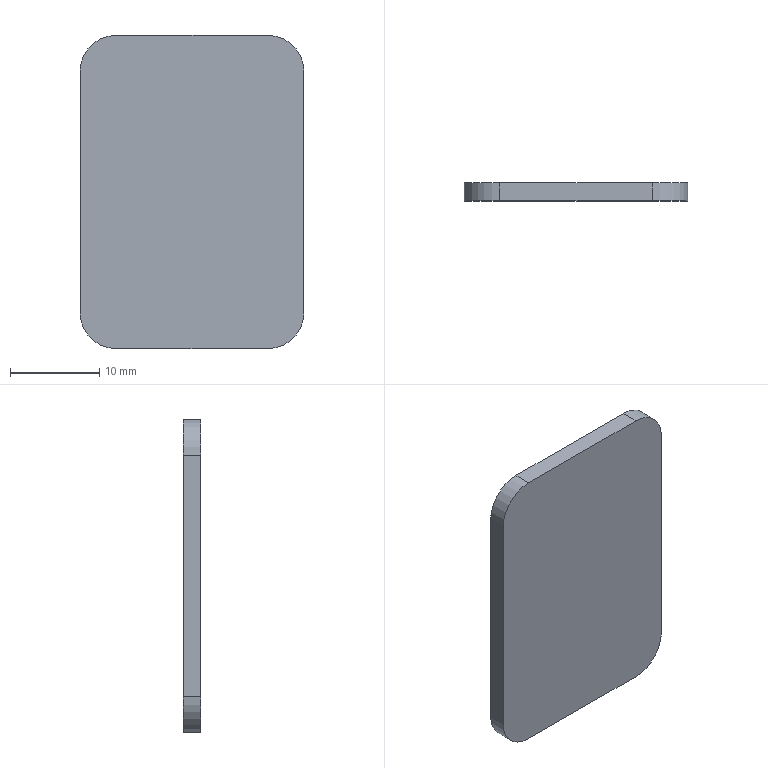Part | SolidWorks | features Extrusion 1 | 1 solid | 10 faces | box 25 x 2 x 35 mm | volume 1723 mm3 | plane 6 | cylinder 4 | commonest cylinder face diameters 8 x4
STEP:
#1=CARTESIAN_POINT('',(12.5,0.,-13.5));
#2=VERTEX_POINT('',#1);
#3=CARTESIAN_POINT('',(8.5,0.,-17.5));
#4=VERTEX_POINT('',#3);
#5=CARTESIAN_POINT('',(8.5,0.,-13.5));
#6=DIRECTION('',(0.,1.,0.));
#7=DIRECTION('',(0.,0.,1.));
#8=AXIS2_PLACEMENT_3D('',#5,#6,#7);
#9=CIRCLE('',#8,4.);
#10=EDGE_CURVE('',#2,#4,#9,.T.);
#11=ORIENTED_EDGE('',*,*,#10,.T.);
#12=CARTESIAN_POINT('',(8.5,2.,-17.5));
#13=VERTEX_POINT('',#12);
#14=CARTESIAN_POINT('',(8.5,2.,-17.5));
#15=DIRECTION('',(0.,-1.,0.));
#16=VECTOR('',#15,1000.);
#17=LINE('',#14,#16);
#18=EDGE_CURVE('',#13,#4,#17,.T.);
#19=ORIENTED_EDGE('',*,*,#18,.F.);
#20=CARTESIAN_POINT('',(12.5,2.,-13.5));
#21=VERTEX_POINT('',#20);
#22=CARTESIAN_POINT('',(8.5,2.,-13.5));
#23=DIRECTION('',(0.,1.,0.));
#24=DIRECTION('',(0.,0.,1.));
#25=AXIS2_PLACEMENT_3D('',#22,#23,#24);
#26=CIRCLE('',#25,4.);
#27=EDGE_CURVE('',#21,#13,#26,.T.);
#28=ORIENTED_EDGE('',*,*,#27,.F.);
#29=CARTESIAN_POINT('',(12.5,2.,-13.5));
#30=DIRECTION('',(0.,-1.,0.));
#31=VECTOR('',#30,1000.);
#32=LINE('',#29,#31);
#33=EDGE_CURVE('',#21,#2,#32,.T.);
#34=ORIENTED_EDGE('',*,*,#33,.T.);
#35=EDGE_LOOP('',(#11,#19,#28,#34));
#36=FACE_OUTER_BOUND('',#35,.T.);
#37=CARTESIAN_POINT('',(8.5,2.,-13.5));
#38=DIRECTION('',(0.,-1.,0.));
#39=DIRECTION('',(0.,0.,-1.));
#40=AXIS2_PLACEMENT_3D('',#37,#38,#39);
#41=CYLINDRICAL_SURFACE('',#40,4.);
#42=ADVANCED_FACE('',(#36),#41,.T.);
#43=CARTESIAN_POINT('',(-8.5,0.,-17.5));
#44=VERTEX_POINT('',#43);
#45=CARTESIAN_POINT('',(8.5,0.,-17.5));
#46=DIRECTION('',(-1.,0.,0.));
#47=VECTOR('',#46,1000.);
#48=LINE('',#45,#47);
#49=EDGE_CURVE('',#4,#44,#48,.T.);
#50=ORIENTED_EDGE('',*,*,#49,.T.);
#51=CARTESIAN_POINT('',(-8.5,2.,-17.5));
#52=VERTEX_POINT('',#51);
#53=CARTESIAN_POINT('',(-8.5,2.,-17.5));
#54=DIRECTION('',(0.,-1.,0.));
#55=VECTOR('',#54,1000.);
#56=LINE('',#53,#55);
#57=EDGE_CURVE('',#52,#44,#56,.T.);
#58=ORIENTED_EDGE('',*,*,#57,.F.);
#59=CARTESIAN_POINT('',(8.5,2.,-17.5));
#60=DIRECTION('',(-1.,0.,0.));
#61=VECTOR('',#60,1000.);
#62=LINE('',#59,#61);
#63=EDGE_CURVE('',#13,#52,#62,.T.);
#64=ORIENTED_EDGE('',*,*,#63,.F.);
#65=ORIENTED_EDGE('',*,*,#18,.T.);
#66=EDGE_LOOP('',(#50,#58,#64,#65));
#67=FACE_OUTER_BOUND('',#66,.T.);
#68=CARTESIAN_POINT('',(8.5,2.,-17.5));
#69=DIRECTION('',(0.,0.,1.));
#70=DIRECTION('',(1.,0.,0.));
#71=AXIS2_PLACEMENT_3D('',#68,#69,#70);
#72=PLANE('',#71);
#73=ADVANCED_FACE('',(#67),#72,.F.);
#74=CARTESIAN_POINT('',(-12.5,0.,-13.5));
#75=VERTEX_POINT('',#74);
#76=CARTESIAN_POINT('',(-8.5,0.,-13.5));
#77=DIRECTION('',(0.,1.,0.));
#78=DIRECTION('',(0.,0.,1.));
#79=AXIS2_PLACEMENT_3D('',#76,#77,#78);
#80=CIRCLE('',#79,4.);
#81=EDGE_CURVE('',#44,#75,#80,.T.);
#82=ORIENTED_EDGE('',*,*,#81,.T.);
#83=CARTESIAN_POINT('',(-12.5,2.,-13.5));
#84=VERTEX_POINT('',#83);
#85=CARTESIAN_POINT('',(-12.5,2.,-13.5));
#86=DIRECTION('',(0.,-1.,0.));
#87=VECTOR('',#86,1000.);
#88=LINE('',#85,#87);
#89=EDGE_CURVE('',#84,#75,#88,.T.);
#90=ORIENTED_EDGE('',*,*,#89,.F.);
#91=CARTESIAN_POINT('',(-8.5,2.,-13.5));
#92=DIRECTION('',(0.,1.,0.));
#93=DIRECTION('',(0.,0.,1.));
#94=AXIS2_PLACEMENT_3D('',#91,#92,#93);
#95=CIRCLE('',#94,4.);
#96=EDGE_CURVE('',#52,#84,#95,.T.);
#97=ORIENTED_EDGE('',*,*,#96,.F.);
#98=ORIENTED_EDGE('',*,*,#57,.T.);
#99=EDGE_LOOP('',(#82,#90,#97,#98));
#100=FACE_OUTER_BOUND('',#99,.T.);
#101=CARTESIAN_POINT('',(-8.5,2.,-13.5));
#102=DIRECTION('',(0.,-1.,0.));
#103=DIRECTION('',(0.,0.,-1.));
#104=AXIS2_PLACEMENT_3D('',#101,#102,#103);
#105=CYLINDRICAL_SURFACE('',#104,4.);
#106=ADVANCED_FACE('',(#100),#105,.T.);
#107=CARTESIAN_POINT('',(-12.5,0.,13.5));
#108=VERTEX_POINT('',#107);
#109=CARTESIAN_POINT('',(-12.5,0.,-13.5));
#110=DIRECTION('',(0.,0.,1.));
#111=VECTOR('',#110,1000.);
#112=LINE('',#109,#111);
#113=EDGE_CURVE('',#75,#108,#112,.T.);
#114=ORIENTED_EDGE('',*,*,#113,.T.);
#115=CARTESIAN_POINT('',(-12.5,2.,13.5));
#116=VERTEX_POINT('',#115);
#117=CARTESIAN_POINT('',(-12.5,2.,13.5));
#118=DIRECTION('',(0.,-1.,0.));
#119=VECTOR('',#118,1000.);
#120=LINE('',#117,#119);
#121=EDGE_CURVE('',#116,#108,#120,.T.);
#122=ORIENTED_EDGE('',*,*,#121,.F.);
#123=CARTESIAN_POINT('',(-12.5,2.,-13.5));
#124=DIRECTION('',(0.,0.,1.));
#125=VECTOR('',#124,1000.);
#126=LINE('',#123,#125);
#127=EDGE_CURVE('',#84,#116,#126,.T.);
#128=ORIENTED_EDGE('',*,*,#127,.F.);
#129=ORIENTED_EDGE('',*,*,#89,.T.);
#130=EDGE_LOOP('',(#114,#122,#128,#129));
#131=FACE_OUTER_BOUND('',#130,.T.);
#132=CARTESIAN_POINT('',(-12.5,2.,-13.5));
#133=DIRECTION('',(1.,0.,0.));
#134=DIRECTION('',(0.,0.,-1.));
#135=AXIS2_PLACEMENT_3D('',#132,#133,#134);
#136=PLANE('',#135);
#137=ADVANCED_FACE('',(#131),#136,.F.);
#138=CARTESIAN_POINT('',(-8.5,0.,17.5));
#139=VERTEX_POINT('',#138);
#140=CARTESIAN_POINT('',(-8.5,0.,13.5));
#141=DIRECTION('',(0.,1.,0.));
#142=DIRECTION('',(0.,0.,1.));
#143=AXIS2_PLACEMENT_3D('',#140,#141,#142);
#144=CIRCLE('',#143,4.);
#145=EDGE_CURVE('',#108,#139,#144,.T.);
#146=ORIENTED_EDGE('',*,*,#145,.T.);
#147=CARTESIAN_POINT('',(-8.5,2.,17.5));
#148=VERTEX_POINT('',#147);
#149=CARTESIAN_POINT('',(-8.5,2.,17.5));
#150=DIRECTION('',(0.,-1.,0.));
#151=VECTOR('',#150,1000.);
#152=LINE('',#149,#151);
#153=EDGE_CURVE('',#148,#139,#152,.T.);
#154=ORIENTED_EDGE('',*,*,#153,.F.);
#155=CARTESIAN_POINT('',(-8.5,2.,13.5));
#156=DIRECTION('',(0.,1.,0.));
#157=DIRECTION('',(0.,0.,1.));
#158=AXIS2_PLACEMENT_3D('',#155,#156,#157);
#159=CIRCLE('',#158,4.);
#160=EDGE_CURVE('',#116,#148,#159,.T.);
#161=ORIENTED_EDGE('',*,*,#160,.F.);
#162=ORIENTED_EDGE('',*,*,#121,.T.);
#163=EDGE_LOOP('',(#146,#154,#161,#162));
#164=FACE_OUTER_BOUND('',#163,.T.);
#165=CARTESIAN_POINT('',(-8.5,2.,13.5));
#166=DIRECTION('',(0.,-1.,0.));
#167=DIRECTION('',(0.,0.,-1.));
#168=AXIS2_PLACEMENT_3D('',#165,#166,#167);
#169=CYLINDRICAL_SURFACE('',#168,4.);
#170=ADVANCED_FACE('',(#164),#169,.T.);
#171=CARTESIAN_POINT('',(8.5,0.,17.5));
#172=VERTEX_POINT('',#171);
#173=CARTESIAN_POINT('',(-8.5,0.,17.5));
#174=DIRECTION('',(1.,0.,0.));
#175=VECTOR('',#174,1000.);
#176=LINE('',#173,#175);
#177=EDGE_CURVE('',#139,#172,#176,.T.);
#178=ORIENTED_EDGE('',*,*,#177,.T.);
#179=CARTESIAN_POINT('',(8.5,2.,17.5));
#180=VERTEX_POINT('',#179);
#181=CARTESIAN_POINT('',(8.5,2.,17.5));
#182=DIRECTION('',(0.,-1.,0.));
#183=VECTOR('',#182,1000.);
#184=LINE('',#181,#183);
#185=EDGE_CURVE('',#180,#172,#184,.T.);
#186=ORIENTED_EDGE('',*,*,#185,.F.);
#187=CARTESIAN_POINT('',(-8.5,2.,17.5));
#188=DIRECTION('',(1.,0.,0.));
#189=VECTOR('',#188,1000.);
#190=LINE('',#187,#189);
#191=EDGE_CURVE('',#148,#180,#190,.T.);
#192=ORIENTED_EDGE('',*,*,#191,.F.);
#193=ORIENTED_EDGE('',*,*,#153,.T.);
#194=EDGE_LOOP('',(#178,#186,#192,#193));
#195=FACE_OUTER_BOUND('',#194,.T.);
#196=CARTESIAN_POINT('',(-8.5,2.,17.5));
#197=DIRECTION('',(0.,0.,-1.));
#198=DIRECTION('',(-1.,0.,0.));
#199=AXIS2_PLACEMENT_3D('',#196,#197,#198);
#200=PLANE('',#199);
#201=ADVANCED_FACE('',(#195),#200,.F.);
#202=CARTESIAN_POINT('',(12.5,0.,13.5));
#203=VERTEX_POINT('',#202);
#204=CARTESIAN_POINT('',(8.5,0.,13.5));
#205=DIRECTION('',(0.,1.,0.));
#206=DIRECTION('',(0.,0.,1.));
#207=AXIS2_PLACEMENT_3D('',#204,#205,#206);
#208=CIRCLE('',#207,4.);
#209=EDGE_CURVE('',#172,#203,#208,.T.);
#210=ORIENTED_EDGE('',*,*,#209,.T.);
#211=CARTESIAN_POINT('',(12.5,2.,13.5));
#212=VERTEX_POINT('',#211);
#213=CARTESIAN_POINT('',(12.5,2.,13.5));
#214=DIRECTION('',(0.,-1.,0.));
#215=VECTOR('',#214,1000.);
#216=LINE('',#213,#215);
#217=EDGE_CURVE('',#212,#203,#216,.T.);
#218=ORIENTED_EDGE('',*,*,#217,.F.);
#219=CARTESIAN_POINT('',(8.5,2.,13.5));
#220=DIRECTION('',(0.,1.,0.));
#221=DIRECTION('',(0.,0.,1.));
#222=AXIS2_PLACEMENT_3D('',#219,#220,#221);
#223=CIRCLE('',#222,4.);
#224=EDGE_CURVE('',#180,#212,#223,.T.);
#225=ORIENTED_EDGE('',*,*,#224,.F.);
#226=ORIENTED_EDGE('',*,*,#185,.T.);
#227=EDGE_LOOP('',(#210,#218,#225,#226));
#228=FACE_OUTER_BOUND('',#227,.T.);
#229=CARTESIAN_POINT('',(8.5,2.,13.5));
#230=DIRECTION('',(0.,-1.,0.));
#231=DIRECTION('',(0.,0.,-1.));
#232=AXIS2_PLACEMENT_3D('',#229,#230,#231);
#233=CYLINDRICAL_SURFACE('',#232,4.);
#234=ADVANCED_FACE('',(#228),#233,.T.);
#235=CARTESIAN_POINT('',(12.5,0.,13.5));
#236=DIRECTION('',(0.,0.,-1.));
#237=VECTOR('',#236,1000.);
#238=LINE('',#235,#237);
#239=EDGE_CURVE('',#203,#2,#238,.T.);
#240=ORIENTED_EDGE('',*,*,#239,.T.);
#241=ORIENTED_EDGE('',*,*,#33,.F.);
#242=CARTESIAN_POINT('',(12.5,2.,13.5));
#243=DIRECTION('',(0.,0.,-1.));
#244=VECTOR('',#243,1000.);
#245=LINE('',#242,#244);
#246=EDGE_CURVE('',#212,#21,#245,.T.);
#247=ORIENTED_EDGE('',*,*,#246,.F.);
#248=ORIENTED_EDGE('',*,*,#217,.T.);
#249=EDGE_LOOP('',(#240,#241,#247,#248));
#250=FACE_OUTER_BOUND('',#249,.T.);
#251=CARTESIAN_POINT('',(12.5,2.,13.5));
#252=DIRECTION('',(-1.,0.,0.));
#253=DIRECTION('',(0.,0.,1.));
#254=AXIS2_PLACEMENT_3D('',#251,#252,#253);
#255=PLANE('',#254);
#256=ADVANCED_FACE('',(#250),#255,.F.);
#257=ORIENTED_EDGE('',*,*,#27,.T.);
#258=ORIENTED_EDGE('',*,*,#63,.T.);
#259=ORIENTED_EDGE('',*,*,#96,.T.);
#260=ORIENTED_EDGE('',*,*,#127,.T.);
#261=ORIENTED_EDGE('',*,*,#160,.T.);
#262=ORIENTED_EDGE('',*,*,#191,.T.);
#263=ORIENTED_EDGE('',*,*,#224,.T.);
#264=ORIENTED_EDGE('',*,*,#246,.T.);
#265=EDGE_LOOP('',(#257,#258,#259,#260,#261,#262,#263,#264));
#266=FACE_OUTER_BOUND('',#265,.T.);
#267=CARTESIAN_POINT('',(8.5,2.,-13.5));
#268=DIRECTION('',(0.,1.,0.));
#269=DIRECTION('',(0.,0.,1.));
#270=AXIS2_PLACEMENT_3D('',#267,#268,#269);
#271=PLANE('',#270);
#272=ADVANCED_FACE('',(#266),#271,.T.);
#273=ORIENTED_EDGE('',*,*,#10,.F.);
#274=ORIENTED_EDGE('',*,*,#239,.F.);
#275=ORIENTED_EDGE('',*,*,#209,.F.);
#276=ORIENTED_EDGE('',*,*,#177,.F.);
#277=ORIENTED_EDGE('',*,*,#145,.F.);
#278=ORIENTED_EDGE('',*,*,#113,.F.);
#279=ORIENTED_EDGE('',*,*,#81,.F.);
#280=ORIENTED_EDGE('',*,*,#49,.F.);
#281=EDGE_LOOP('',(#273,#274,#275,#276,#277,#278,#279,#280));
#282=FACE_OUTER_BOUND('',#281,.T.);
#283=CARTESIAN_POINT('',(8.5,0.,-13.5));
#284=DIRECTION('',(0.,1.,0.));
#285=DIRECTION('',(0.,0.,1.));
#286=AXIS2_PLACEMENT_3D('',#283,#284,#285);
#287=PLANE('',#286);
#288=ADVANCED_FACE('',(#282),#287,.F.);
#289=CLOSED_SHELL('',(#42,#73,#106,#137,#170,#201,#234,#256,#272,#288));
#290=MANIFOLD_SOLID_BREP('',#289);
#291=CARTESIAN_POINT('',(0.,0.,0.));
#292=DIRECTION('',(0.,0.,1.));
#293=DIRECTION('',(1.,0.,0.));
#294=AXIS2_PLACEMENT_3D('',#291,#292,#293);
#295=(LENGTH_UNIT()NAMED_UNIT(*)SI_UNIT(.MILLI.,.METRE.));
#296=UNCERTAINTY_MEASURE_WITH_UNIT(LENGTH_MEASURE(0.00001),#295,'','');
#297=(NAMED_UNIT(*)PLANE_ANGLE_UNIT()SI_UNIT($,.RADIAN.));
#298=(NAMED_UNIT(*)SI_UNIT($,.STERADIAN.)SOLID_ANGLE_UNIT());
#299=(GEOMETRIC_REPRESENTATION_CONTEXT(3)GLOBAL_UNCERTAINTY_ASSIGNED_CONTEXT((#296))GLOBAL_UNIT_ASSIGNED_CONTEXT((#295,#297,#298))REPRESENTATION_CONTEXT('',''));
#300=ADVANCED_BREP_SHAPE_REPRESENTATION('',(#290,#294),#299);